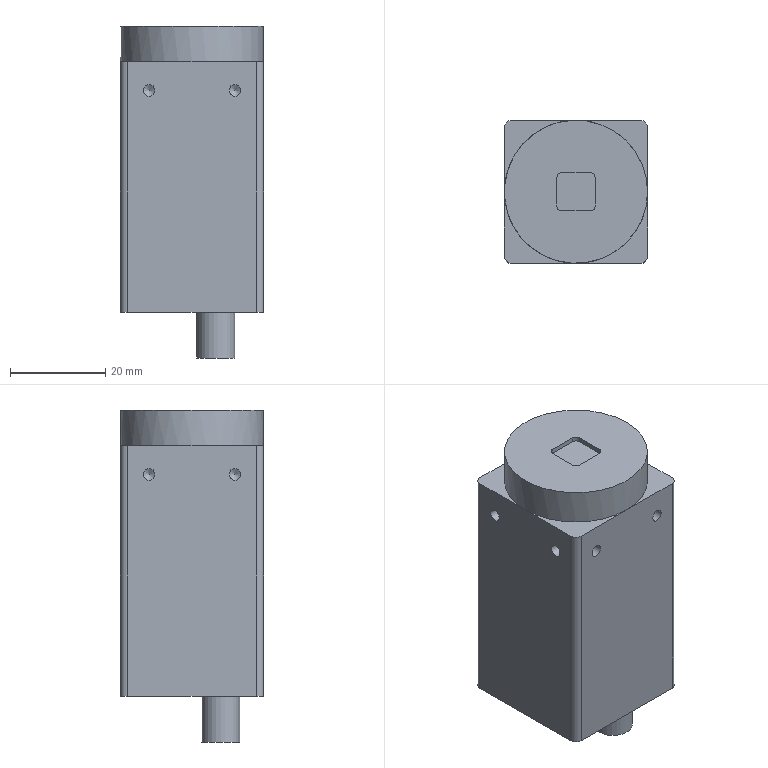Part | NX | 1 solid | 56 faces | box 30 x 30 x 69.6 mm | volume 52533 mm3 | cylinder 29 | plane 16 | cone 11 | commonest cylinder face diameters 2.5 x16 2 x4 3 x4 2.05 x3 8 x1 30 x1
STEP:
#1=CARTESIAN_POINT('',(9.,-15.,45.25));
#2=VERTEX_POINT('',#1);
#3=CARTESIAN_POINT('',(9.,-15.,46.5));
#4=DIRECTION('',(0.,-1.,0.));
#5=DIRECTION('',(0.,0.,-1.));
#6=AXIS2_PLACEMENT_3D('',#3,#4,#5);
#7=CIRCLE('',#6,1.25);
#8=EDGE_CURVE('',#2,#2,#7,.T.);
#9=ORIENTED_EDGE('',*,*,#8,.T.);
#10=EDGE_LOOP('',(#9));
#11=FACE_BOUND('',#10,.T.);
#12=CARTESIAN_POINT('',(9.,-9.,47.75));
#13=VERTEX_POINT('',#12);
#14=CARTESIAN_POINT('',(9.,-9.,45.25));
#15=VERTEX_POINT('',#14);
#16=CARTESIAN_POINT('',(9.,-9.,46.5));
#17=DIRECTION('',(-0.7071,-0.7071,0.));
#18=DIRECTION('',(0.7071,-0.7071,0.));
#19=AXIS2_PLACEMENT_3D('',#16,#17,#18);
#20=ELLIPSE('',#19,1.768,1.25);
#21=EDGE_CURVE('',#13,#15,#20,.F.);
#22=ORIENTED_EDGE('',*,*,#21,.T.);
#23=CARTESIAN_POINT('',(9.,-9.,46.5));
#24=DIRECTION('',(0.7071,-0.7071,0.));
#25=DIRECTION('',(-0.7071,-0.7071,0.));
#26=AXIS2_PLACEMENT_3D('',#23,#24,#25);
#27=ELLIPSE('',#26,1.768,1.25);
#28=EDGE_CURVE('',#15,#13,#27,.F.);
#29=ORIENTED_EDGE('',*,*,#28,.T.);
#30=EDGE_LOOP('',(#22,#29));
#31=FACE_BOUND('',#30,.T.);
#32=CARTESIAN_POINT('',(9.,-15.,46.5));
#33=DIRECTION('',(0.,-1.,0.));
#34=DIRECTION('',(0.,0.,-1.));
#35=AXIS2_PLACEMENT_3D('',#32,#33,#34);
#36=CYLINDRICAL_SURFACE('',#35,1.25);
#37=ADVANCED_FACE('',(#11,#31),#36,.F.);
#38=CARTESIAN_POINT('',(9.,15.,47.75));
#39=VERTEX_POINT('',#38);
#40=CARTESIAN_POINT('',(9.,15.,46.5));
#41=DIRECTION('',(0.,1.,0.));
#42=DIRECTION('',(0.,0.,1.));
#43=AXIS2_PLACEMENT_3D('',#40,#41,#42);
#44=CIRCLE('',#43,1.25);
#45=EDGE_CURVE('',#39,#39,#44,.T.);
#46=ORIENTED_EDGE('',*,*,#45,.T.);
#47=EDGE_LOOP('',(#46));
#48=FACE_BOUND('',#47,.T.);
#49=CARTESIAN_POINT('',(9.,9.,45.25));
#50=VERTEX_POINT('',#49);
#51=CARTESIAN_POINT('',(9.,9.,47.75));
#52=VERTEX_POINT('',#51);
#53=CARTESIAN_POINT('',(9.,9.,46.5));
#54=DIRECTION('',(-0.7071,0.7071,0.));
#55=DIRECTION('',(0.7071,0.7071,0.));
#56=AXIS2_PLACEMENT_3D('',#53,#54,#55);
#57=ELLIPSE('',#56,1.768,1.25);
#58=EDGE_CURVE('',#50,#52,#57,.F.);
#59=ORIENTED_EDGE('',*,*,#58,.T.);
#60=CARTESIAN_POINT('',(9.,9.,46.5));
#61=DIRECTION('',(0.7071,0.7071,0.));
#62=DIRECTION('',(-0.7071,0.7071,0.));
#63=AXIS2_PLACEMENT_3D('',#60,#61,#62);
#64=ELLIPSE('',#63,1.768,1.25);
#65=EDGE_CURVE('',#52,#50,#64,.F.);
#66=ORIENTED_EDGE('',*,*,#65,.T.);
#67=EDGE_LOOP('',(#59,#66));
#68=FACE_BOUND('',#67,.T.);
#69=CARTESIAN_POINT('',(9.,15.,46.5));
#70=DIRECTION('',(0.,1.,0.));
#71=DIRECTION('',(0.,0.,1.));
#72=AXIS2_PLACEMENT_3D('',#69,#70,#71);
#73=CYLINDRICAL_SURFACE('',#72,1.25);
#74=ADVANCED_FACE('',(#48,#68),#73,.F.);
#75=CARTESIAN_POINT('',(-15.,9.,47.75));
#76=VERTEX_POINT('',#75);
#77=CARTESIAN_POINT('',(-15.,9.,46.5));
#78=DIRECTION('',(-1.,0.,0.));
#79=DIRECTION('',(0.,0.,1.));
#80=AXIS2_PLACEMENT_3D('',#77,#78,#79);
#81=CIRCLE('',#80,1.25);
#82=EDGE_CURVE('',#76,#76,#81,.T.);
#83=ORIENTED_EDGE('',*,*,#82,.T.);
#84=EDGE_LOOP('',(#83));
#85=FACE_BOUND('',#84,.T.);
#86=CARTESIAN_POINT('',(-9.,9.,45.25));
#87=VERTEX_POINT('',#86);
#88=CARTESIAN_POINT('',(-9.,9.,47.75));
#89=VERTEX_POINT('',#88);
#90=CARTESIAN_POINT('',(-9.,9.,46.5));
#91=DIRECTION('',(-0.7071,-0.7071,0.));
#92=DIRECTION('',(-0.7071,0.7071,0.));
#93=AXIS2_PLACEMENT_3D('',#90,#91,#92);
#94=ELLIPSE('',#93,1.768,1.25);
#95=EDGE_CURVE('',#87,#89,#94,.F.);
#96=ORIENTED_EDGE('',*,*,#95,.T.);
#97=CARTESIAN_POINT('',(-9.,9.,46.5));
#98=DIRECTION('',(-0.7071,0.7071,0.));
#99=DIRECTION('',(-0.7071,-0.7071,0.));
#100=AXIS2_PLACEMENT_3D('',#97,#98,#99);
#101=ELLIPSE('',#100,1.768,1.25);
#102=EDGE_CURVE('',#89,#87,#101,.F.);
#103=ORIENTED_EDGE('',*,*,#102,.T.);
#104=EDGE_LOOP('',(#96,#103));
#105=FACE_BOUND('',#104,.T.);
#106=CARTESIAN_POINT('',(-15.,9.,46.5));
#107=DIRECTION('',(-1.,0.,0.));
#108=DIRECTION('',(0.,0.,1.));
#109=AXIS2_PLACEMENT_3D('',#106,#107,#108);
#110=CYLINDRICAL_SURFACE('',#109,1.25);
#111=ADVANCED_FACE('',(#85,#105),#110,.F.);
#112=CARTESIAN_POINT('',(-9.,-15.,45.25));
#113=VERTEX_POINT('',#112);
#114=CARTESIAN_POINT('',(-9.,-15.,46.5));
#115=DIRECTION('',(0.,-1.,0.));
#116=DIRECTION('',(0.,0.,-1.));
#117=AXIS2_PLACEMENT_3D('',#114,#115,#116);
#118=CIRCLE('',#117,1.25);
#119=EDGE_CURVE('',#113,#113,#118,.T.);
#120=ORIENTED_EDGE('',*,*,#119,.T.);
#121=EDGE_LOOP('',(#120));
#122=FACE_BOUND('',#121,.T.);
#123=CARTESIAN_POINT('',(-9.,-9.,45.25));
#124=VERTEX_POINT('',#123);
#125=CARTESIAN_POINT('',(-9.,-9.,47.75));
#126=VERTEX_POINT('',#125);
#127=CARTESIAN_POINT('',(-9.,-9.,46.5));
#128=DIRECTION('',(0.7071,-0.7071,0.));
#129=DIRECTION('',(-0.7071,-0.7071,0.));
#130=AXIS2_PLACEMENT_3D('',#127,#128,#129);
#131=ELLIPSE('',#130,1.768,1.25);
#132=EDGE_CURVE('',#124,#126,#131,.F.);
#133=ORIENTED_EDGE('',*,*,#132,.T.);
#134=CARTESIAN_POINT('',(-9.,-9.,46.5));
#135=DIRECTION('',(-0.7071,-0.7071,0.));
#136=DIRECTION('',(0.7071,-0.7071,0.));
#137=AXIS2_PLACEMENT_3D('',#134,#135,#136);
#138=ELLIPSE('',#137,1.768,1.25);
#139=EDGE_CURVE('',#126,#124,#138,.F.);
#140=ORIENTED_EDGE('',*,*,#139,.T.);
#141=EDGE_LOOP('',(#133,#140));
#142=FACE_BOUND('',#141,.T.);
#143=CARTESIAN_POINT('',(-9.,-15.,46.5));
#144=DIRECTION('',(0.,-1.,0.));
#145=DIRECTION('',(0.,0.,-1.));
#146=AXIS2_PLACEMENT_3D('',#143,#144,#145);
#147=CYLINDRICAL_SURFACE('',#146,1.25);
#148=ADVANCED_FACE('',(#122,#142),#147,.F.);
#149=CARTESIAN_POINT('',(15.,0.,60.));
#150=VERTEX_POINT('',#149);
#151=CARTESIAN_POINT('',(0.,0.,60.));
#152=DIRECTION('',(0.,0.,1.));
#153=DIRECTION('',(1.,0.,0.));
#154=AXIS2_PLACEMENT_3D('',#151,#152,#153);
#155=CIRCLE('',#154,15.);
#156=EDGE_CURVE('',#150,#150,#155,.T.);
#157=ORIENTED_EDGE('',*,*,#156,.T.);
#158=EDGE_LOOP('',(#157));
#159=FACE_BOUND('',#158,.T.);
#160=CARTESIAN_POINT('',(-4.,-3.,60.));
#161=VERTEX_POINT('',#160);
#162=CARTESIAN_POINT('',(-4.,3.,60.));
#163=VERTEX_POINT('',#162);
#164=CARTESIAN_POINT('',(-4.,3.,60.));
#165=DIRECTION('',(0.,1.,0.));
#166=VECTOR('',#165,1000.);
#167=LINE('',#164,#166);
#168=EDGE_CURVE('',#161,#163,#167,.T.);
#169=ORIENTED_EDGE('',*,*,#168,.T.);
#170=CARTESIAN_POINT('',(-3.,4.,60.));
#171=VERTEX_POINT('',#170);
#172=CARTESIAN_POINT('',(-3.,3.,60.));
#173=DIRECTION('',(0.,0.,-1.));
#174=DIRECTION('',(-1.,0.,0.));
#175=AXIS2_PLACEMENT_3D('',#172,#173,#174);
#176=CIRCLE('',#175,1.);
#177=EDGE_CURVE('',#163,#171,#176,.T.);
#178=ORIENTED_EDGE('',*,*,#177,.T.);
#179=CARTESIAN_POINT('',(3.,4.,60.));
#180=VERTEX_POINT('',#179);
#181=CARTESIAN_POINT('',(3.,4.,60.));
#182=DIRECTION('',(1.,0.,0.));
#183=VECTOR('',#182,1000.);
#184=LINE('',#181,#183);
#185=EDGE_CURVE('',#171,#180,#184,.T.);
#186=ORIENTED_EDGE('',*,*,#185,.T.);
#187=CARTESIAN_POINT('',(4.,3.,60.));
#188=VERTEX_POINT('',#187);
#189=CARTESIAN_POINT('',(3.,3.,60.));
#190=DIRECTION('',(0.,0.,-1.));
#191=DIRECTION('',(-1.,0.,0.));
#192=AXIS2_PLACEMENT_3D('',#189,#190,#191);
#193=CIRCLE('',#192,1.);
#194=EDGE_CURVE('',#180,#188,#193,.T.);
#195=ORIENTED_EDGE('',*,*,#194,.T.);
#196=CARTESIAN_POINT('',(4.,-3.,60.));
#197=VERTEX_POINT('',#196);
#198=CARTESIAN_POINT('',(4.,3.,60.));
#199=DIRECTION('',(0.,-1.,0.));
#200=VECTOR('',#199,1000.);
#201=LINE('',#198,#200);
#202=EDGE_CURVE('',#188,#197,#201,.T.);
#203=ORIENTED_EDGE('',*,*,#202,.T.);
#204=CARTESIAN_POINT('',(3.,-4.,60.));
#205=VERTEX_POINT('',#204);
#206=CARTESIAN_POINT('',(3.,-3.,60.));
#207=DIRECTION('',(0.,0.,-1.));
#208=DIRECTION('',(-1.,0.,0.));
#209=AXIS2_PLACEMENT_3D('',#206,#207,#208);
#210=CIRCLE('',#209,1.);
#211=EDGE_CURVE('',#197,#205,#210,.T.);
#212=ORIENTED_EDGE('',*,*,#211,.T.);
#213=CARTESIAN_POINT('',(-3.,-4.,60.));
#214=VERTEX_POINT('',#213);
#215=CARTESIAN_POINT('',(3.,-4.,60.));
#216=DIRECTION('',(-1.,0.,0.));
#217=VECTOR('',#216,1000.);
#218=LINE('',#215,#217);
#219=EDGE_CURVE('',#205,#214,#218,.T.);
#220=ORIENTED_EDGE('',*,*,#219,.T.);
#221=CARTESIAN_POINT('',(-3.,-3.,60.));
#222=DIRECTION('',(0.,0.,-1.));
#223=DIRECTION('',(-1.,0.,0.));
#224=AXIS2_PLACEMENT_3D('',#221,#222,#223);
#225=CIRCLE('',#224,1.);
#226=EDGE_CURVE('',#214,#161,#225,.T.);
#227=ORIENTED_EDGE('',*,*,#226,.T.);
#228=EDGE_LOOP('',(#169,#178,#186,#195,#203,#212,#220,#227));
#229=FACE_BOUND('',#228,.T.);
#230=CARTESIAN_POINT('',(0.,0.,60.));
#231=DIRECTION('',(0.,0.,1.));
#232=DIRECTION('',(1.,0.,0.));
#233=AXIS2_PLACEMENT_3D('',#230,#231,#232);
#234=PLANE('',#233);
#235=ADVANCED_FACE('',(#159,#229),#234,.T.);
#236=CARTESIAN_POINT('',(13.5,-15.,0.));
#237=VERTEX_POINT('',#236);
#238=CARTESIAN_POINT('',(15.,-13.5,0.));
#239=VERTEX_POINT('',#238);
#240=CARTESIAN_POINT('',(13.5,-13.5,0.));
#241=DIRECTION('',(0.,0.,1.));
#242=DIRECTION('',(1.,0.,0.));
#243=AXIS2_PLACEMENT_3D('',#240,#241,#242);
#244=CIRCLE('',#243,1.5);
#245=EDGE_CURVE('',#237,#239,#244,.T.);
#246=ORIENTED_EDGE('',*,*,#245,.F.);
#247=CARTESIAN_POINT('',(-13.5,-15.,0.));
#248=VERTEX_POINT('',#247);
#249=CARTESIAN_POINT('',(-13.5,-15.,0.));
#250=DIRECTION('',(1.,0.,0.));
#251=VECTOR('',#250,1000.);
#252=LINE('',#249,#251);
#253=EDGE_CURVE('',#248,#237,#252,.T.);
#254=ORIENTED_EDGE('',*,*,#253,.F.);
#255=CARTESIAN_POINT('',(-15.,-13.5,0.));
#256=VERTEX_POINT('',#255);
#257=CARTESIAN_POINT('',(-13.5,-13.5,0.));
#258=DIRECTION('',(0.,0.,1.));
#259=DIRECTION('',(1.,0.,0.));
#260=AXIS2_PLACEMENT_3D('',#257,#258,#259);
#261=CIRCLE('',#260,1.5);
#262=EDGE_CURVE('',#256,#248,#261,.T.);
#263=ORIENTED_EDGE('',*,*,#262,.F.);
#264=CARTESIAN_POINT('',(-15.,13.5,0.));
#265=VERTEX_POINT('',#264);
#266=CARTESIAN_POINT('',(-15.,-13.5,0.));
#267=DIRECTION('',(0.,-1.,0.));
#268=VECTOR('',#267,1000.);
#269=LINE('',#266,#268);
#270=EDGE_CURVE('',#265,#256,#269,.T.);
#271=ORIENTED_EDGE('',*,*,#270,.F.);
#272=CARTESIAN_POINT('',(-13.5,15.,0.));
#273=VERTEX_POINT('',#272);
#274=CARTESIAN_POINT('',(-13.5,13.5,0.));
#275=DIRECTION('',(0.,0.,1.));
#276=DIRECTION('',(1.,0.,0.));
#277=AXIS2_PLACEMENT_3D('',#274,#275,#276);
#278=CIRCLE('',#277,1.5);
#279=EDGE_CURVE('',#273,#265,#278,.T.);
#280=ORIENTED_EDGE('',*,*,#279,.F.);
#281=CARTESIAN_POINT('',(13.5,15.,0.));
#282=VERTEX_POINT('',#281);
#283=CARTESIAN_POINT('',(-13.5,15.,0.));
#284=DIRECTION('',(-1.,0.,0.));
#285=VECTOR('',#284,1000.);
#286=LINE('',#283,#285);
#287=EDGE_CURVE('',#282,#273,#286,.T.);
#288=ORIENTED_EDGE('',*,*,#287,.F.);
#289=CARTESIAN_POINT('',(15.,13.5,0.));
#290=VERTEX_POINT('',#289);
#291=CARTESIAN_POINT('',(13.5,13.5,0.));
#292=DIRECTION('',(0.,0.,1.));
#293=DIRECTION('',(1.,0.,0.));
#294=AXIS2_PLACEMENT_3D('',#291,#292,#293);
#295=CIRCLE('',#294,1.5);
#296=EDGE_CURVE('',#290,#282,#295,.T.);
#297=ORIENTED_EDGE('',*,*,#296,.F.);
#298=CARTESIAN_POINT('',(15.,-13.5,0.));
#299=DIRECTION('',(0.,1.,0.));
#300=VECTOR('',#299,1000.);
#301=LINE('',#298,#300);
#302=EDGE_CURVE('',#239,#290,#301,.T.);
#303=ORIENTED_EDGE('',*,*,#302,.F.);
#304=EDGE_LOOP('',(#246,#254,#263,#271,#280,#288,#297,#303));
#305=FACE_BOUND('',#304,.T.);
#306=CARTESIAN_POINT('',(9.,-6.,0.));
#307=VERTEX_POINT('',#306);
#308=CARTESIAN_POINT('',(5.,-6.,0.));
#309=DIRECTION('',(0.,0.,1.));
#310=DIRECTION('',(1.,0.,0.));
#311=AXIS2_PLACEMENT_3D('',#308,#309,#310);
#312=CIRCLE('',#311,4.);
#313=EDGE_CURVE('',#307,#307,#312,.F.);
#314=ORIENTED_EDGE('',*,*,#313,.F.);
#315=EDGE_LOOP('',(#314));
#316=FACE_BOUND('',#315,.T.);
#317=CARTESIAN_POINT('',(13.5,-13.5,0.));
#318=DIRECTION('',(0.,0.,1.));
#319=DIRECTION('',(1.,0.,0.));
#320=AXIS2_PLACEMENT_3D('',#317,#318,#319);
#321=PLANE('',#320);
#322=ADVANCED_FACE('',(#305,#316),#321,.F.);
#323=CARTESIAN_POINT('',(15.,0.,52.5));
#324=VERTEX_POINT('',#323);
#325=CARTESIAN_POINT('',(0.,15.,52.5));
#326=VERTEX_POINT('',#325);
#327=CARTESIAN_POINT('',(0.,0.,52.5));
#328=DIRECTION('',(0.,0.,1.));
#329=DIRECTION('',(1.,0.,0.));
#330=AXIS2_PLACEMENT_3D('',#327,#328,#329);
#331=CIRCLE('',#330,15.);
#332=EDGE_CURVE('',#324,#326,#331,.T.);
#333=ORIENTED_EDGE('',*,*,#332,.F.);
#334=CARTESIAN_POINT('',(15.,13.5,52.5));
#335=VERTEX_POINT('',#334);
#336=CARTESIAN_POINT('',(15.,-13.5,52.5));
#337=DIRECTION('',(0.,1.,0.));
#338=VECTOR('',#337,1000.);
#339=LINE('',#336,#338);
#340=EDGE_CURVE('',#324,#335,#339,.T.);
#341=ORIENTED_EDGE('',*,*,#340,.T.);
#342=CARTESIAN_POINT('',(13.5,15.,52.5));
#343=VERTEX_POINT('',#342);
#344=CARTESIAN_POINT('',(13.5,13.5,52.5));
#345=DIRECTION('',(0.,0.,1.));
#346=DIRECTION('',(1.,0.,0.));
#347=AXIS2_PLACEMENT_3D('',#344,#345,#346);
#348=CIRCLE('',#347,1.5);
#349=EDGE_CURVE('',#335,#343,#348,.T.);
#350=ORIENTED_EDGE('',*,*,#349,.T.);
#351=CARTESIAN_POINT('',(-13.5,15.,52.5));
#352=DIRECTION('',(-1.,0.,0.));
#353=VECTOR('',#352,1000.);
#354=LINE('',#351,#353);
#355=EDGE_CURVE('',#343,#326,#354,.T.);
#356=ORIENTED_EDGE('',*,*,#355,.T.);
#357=EDGE_LOOP('',(#333,#341,#350,#356));
#358=FACE_BOUND('',#357,.T.);
#359=CARTESIAN_POINT('',(13.5,-13.5,52.5));
#360=DIRECTION('',(0.,0.,1.));
#361=DIRECTION('',(1.,0.,0.));
#362=AXIS2_PLACEMENT_3D('',#359,#360,#361);
#363=PLANE('',#362);
#364=ADVANCED_FACE('',(#358),#363,.T.);
#365=CARTESIAN_POINT('',(-15.,0.,52.5));
#366=VERTEX_POINT('',#365);
#367=CARTESIAN_POINT('',(0.,0.,52.5));
#368=DIRECTION('',(0.,0.,1.));
#369=DIRECTION('',(1.,0.,0.));
#370=AXIS2_PLACEMENT_3D('',#367,#368,#369);
#371=CIRCLE('',#370,15.);
#372=EDGE_CURVE('',#326,#366,#371,.T.);
#373=ORIENTED_EDGE('',*,*,#372,.F.);
#374=CARTESIAN_POINT('',(-13.5,15.,52.5));
#375=VERTEX_POINT('',#374);
#376=CARTESIAN_POINT('',(-13.5,15.,52.5));
#377=DIRECTION('',(-1.,0.,0.));
#378=VECTOR('',#377,1000.);
#379=LINE('',#376,#378);
#380=EDGE_CURVE('',#326,#375,#379,.T.);
#381=ORIENTED_EDGE('',*,*,#380,.T.);
#382=CARTESIAN_POINT('',(-15.,13.5,52.5));
#383=VERTEX_POINT('',#382);
#384=CARTESIAN_POINT('',(-13.5,13.5,52.5));
#385=DIRECTION('',(0.,0.,1.));
#386=DIRECTION('',(1.,0.,0.));
#387=AXIS2_PLACEMENT_3D('',#384,#385,#386);
#388=CIRCLE('',#387,1.5);
#389=EDGE_CURVE('',#375,#383,#388,.T.);
#390=ORIENTED_EDGE('',*,*,#389,.T.);
#391=CARTESIAN_POINT('',(-15.,-13.5,52.5));
#392=DIRECTION('',(0.,-1.,0.));
#393=VECTOR('',#392,1000.);
#394=LINE('',#391,#393);
#395=EDGE_CURVE('',#383,#366,#394,.T.);
#396=ORIENTED_EDGE('',*,*,#395,.T.);
#397=EDGE_LOOP('',(#373,#381,#390,#396));
#398=FACE_BOUND('',#397,.T.);
#399=CARTESIAN_POINT('',(13.5,-13.5,52.5));
#400=DIRECTION('',(0.,0.,1.));
#401=DIRECTION('',(1.,0.,0.));
#402=AXIS2_PLACEMENT_3D('',#399,#400,#401);
#403=PLANE('',#402);
#404=ADVANCED_FACE('',(#398),#403,.T.);
#405=CARTESIAN_POINT('',(0.,-15.,52.5));
#406=VERTEX_POINT('',#405);
#407=CARTESIAN_POINT('',(0.,0.,52.5));
#408=DIRECTION('',(0.,0.,1.));
#409=DIRECTION('',(1.,0.,0.));
#410=AXIS2_PLACEMENT_3D('',#407,#408,#409);
#411=CIRCLE('',#410,15.);
#412=EDGE_CURVE('',#366,#406,#411,.T.);
#413=ORIENTED_EDGE('',*,*,#412,.F.);
#414=CARTESIAN_POINT('',(-15.,-13.5,52.5));
#415=VERTEX_POINT('',#414);
#416=CARTESIAN_POINT('',(-15.,-13.5,52.5));
#417=DIRECTION('',(0.,-1.,0.));
#418=VECTOR('',#417,1000.);
#419=LINE('',#416,#418);
#420=EDGE_CURVE('',#366,#415,#419,.T.);
#421=ORIENTED_EDGE('',*,*,#420,.T.);
#422=CARTESIAN_POINT('',(-13.5,-15.,52.5));
#423=VERTEX_POINT('',#422);
#424=CARTESIAN_POINT('',(-13.5,-13.5,52.5));
#425=DIRECTION('',(0.,0.,1.));
#426=DIRECTION('',(1.,0.,0.));
#427=AXIS2_PLACEMENT_3D('',#424,#425,#426);
#428=CIRCLE('',#427,1.5);
#429=EDGE_CURVE('',#415,#423,#428,.T.);
#430=ORIENTED_EDGE('',*,*,#429,.T.);
#431=CARTESIAN_POINT('',(-13.5,-15.,52.5));
#432=DIRECTION('',(1.,0.,0.));
#433=VECTOR('',#432,1000.);
#434=LINE('',#431,#433);
#435=EDGE_CURVE('',#423,#406,#434,.T.);
#436=ORIENTED_EDGE('',*,*,#435,.T.);
#437=EDGE_LOOP('',(#413,#421,#430,#436));
#438=FACE_BOUND('',#437,.T.);
#439=CARTESIAN_POINT('',(13.5,-13.5,52.5));
#440=DIRECTION('',(0.,0.,1.));
#441=DIRECTION('',(1.,0.,0.));
#442=AXIS2_PLACEMENT_3D('',#439,#440,#441);
#443=PLANE('',#442);
#444=ADVANCED_FACE('',(#438),#443,.T.);
#445=ORIENTED_EDGE('',*,*,#245,.T.);
#446=CARTESIAN_POINT('',(15.,-13.5,52.5));
#447=VERTEX_POINT('',#446);
#448=CARTESIAN_POINT('',(15.,-13.5,52.5));
#449=DIRECTION('',(0.,0.,-1.));
#450=VECTOR('',#449,1000.);
#451=LINE('',#448,#450);
#452=EDGE_CURVE('',#447,#239,#451,.T.);
#453=ORIENTED_EDGE('',*,*,#452,.F.);
#454=CARTESIAN_POINT('',(13.5,-15.,52.5));
#455=VERTEX_POINT('',#454);
#456=CARTESIAN_POINT('',(13.5,-13.5,52.5));
#457=DIRECTION('',(0.,0.,1.));
#458=DIRECTION('',(1.,0.,0.));
#459=AXIS2_PLACEMENT_3D('',#456,#457,#458);
#460=CIRCLE('',#459,1.5);
#461=EDGE_CURVE('',#455,#447,#460,.T.);
#462=ORIENTED_EDGE('',*,*,#461,.F.);
#463=CARTESIAN_POINT('',(13.5,-15.,52.5));
#464=DIRECTION('',(0.,0.,-1.));
#465=VECTOR('',#464,1000.);
#466=LINE('',#463,#465);
#467=EDGE_CURVE('',#455,#237,#466,.T.);
#468=ORIENTED_EDGE('',*,*,#467,.T.);
#469=EDGE_LOOP('',(#445,#453,#462,#468));
#470=FACE_BOUND('',#469,.T.);
#471=CARTESIAN_POINT('',(13.5,-13.5,52.5));
#472=DIRECTION('',(0.,0.,-1.));
#473=DIRECTION('',(-1.,0.,0.));
#474=AXIS2_PLACEMENT_3D('',#471,#472,#473);
#475=CYLINDRICAL_SURFACE('',#474,1.5);
#476=ADVANCED_FACE('',(#470),#475,.T.);
#477=CARTESIAN_POINT('',(15.,-9.,45.25));
#478=VERTEX_POINT('',#477);
#479=CARTESIAN_POINT('',(15.,-9.,46.5));
#480=DIRECTION('',(1.,0.,0.));
#481=DIRECTION('',(0.,0.,-1.));
#482=AXIS2_PLACEMENT_3D('',#479,#480,#481);
#483=CIRCLE('',#482,1.25);
#484=EDGE_CURVE('',#478,#478,#483,.T.);
#485=ORIENTED_EDGE('',*,*,#484,.F.);
#486=EDGE_LOOP('',(#485));
#487=FACE_BOUND('',#486,.T.);
#488=CARTESIAN_POINT('',(15.,9.,45.25));
#489=VERTEX_POINT('',#488);
#490=CARTESIAN_POINT('',(15.,9.,46.5));
#491=DIRECTION('',(1.,0.,0.));
#492=DIRECTION('',(0.,0.,-1.));
#493=AXIS2_PLACEMENT_3D('',#490,#491,#492);
#494=CIRCLE('',#493,1.25);
#495=EDGE_CURVE('',#489,#489,#494,.T.);
#496=ORIENTED_EDGE('',*,*,#495,.F.);
#497=EDGE_LOOP('',(#496));
#498=FACE_BOUND('',#497,.T.);
#499=ORIENTED_EDGE('',*,*,#302,.T.);
#500=CARTESIAN_POINT('',(15.,13.5,52.5));
#501=DIRECTION('',(0.,0.,-1.));
#502=VECTOR('',#501,1000.);
#503=LINE('',#500,#502);
#504=EDGE_CURVE('',#335,#290,#503,.T.);
#505=ORIENTED_EDGE('',*,*,#504,.F.);
#506=ORIENTED_EDGE('',*,*,#340,.F.);
#507=CARTESIAN_POINT('',(15.,-13.5,52.5));
#508=DIRECTION('',(0.,1.,0.));
#509=VECTOR('',#508,1000.);
#510=LINE('',#507,#509);
#511=EDGE_CURVE('',#447,#324,#510,.T.);
#512=ORIENTED_EDGE('',*,*,#511,.F.);
#513=ORIENTED_EDGE('',*,*,#452,.T.);
#514=EDGE_LOOP('',(#499,#505,#506,#512,#513));
#515=FACE_BOUND('',#514,.T.);
#516=CARTESIAN_POINT('',(15.,-13.5,52.5));
#517=DIRECTION('',(-1.,0.,0.));
#518=DIRECTION('',(0.,-1.,0.));
#519=AXIS2_PLACEMENT_3D('',#516,#517,#518);
#520=PLANE('',#519);
#521=ADVANCED_FACE('',(#487,#498,#515),#520,.F.);
#522=ORIENTED_EDGE('',*,*,#296,.T.);
#523=CARTESIAN_POINT('',(13.5,15.,52.5));
#524=DIRECTION('',(0.,0.,-1.));
#525=VECTOR('',#524,1000.);
#526=LINE('',#523,#525);
#527=EDGE_CURVE('',#343,#282,#526,.T.);
#528=ORIENTED_EDGE('',*,*,#527,.F.);
#529=ORIENTED_EDGE('',*,*,#349,.F.);
#530=ORIENTED_EDGE('',*,*,#504,.T.);
#531=EDGE_LOOP('',(#522,#528,#529,#530));
#532=FACE_BOUND('',#531,.T.);
#533=CARTESIAN_POINT('',(13.5,13.5,52.5));
#534=DIRECTION('',(0.,0.,-1.));
#535=DIRECTION('',(-1.,0.,0.));
#536=AXIS2_PLACEMENT_3D('',#533,#534,#535);
#537=CYLINDRICAL_SURFACE('',#536,1.5);
#538=ADVANCED_FACE('',(#532),#537,.T.);
#539=CARTESIAN_POINT('',(0.,15.,47.525));
#540=VERTEX_POINT('',#539);
#541=CARTESIAN_POINT('',(0.,15.,46.5));
#542=DIRECTION('',(0.,1.,0.));
#543=DIRECTION('',(0.,0.,1.));
#544=AXIS2_PLACEMENT_3D('',#541,#542,#543);
#545=CIRCLE('',#544,1.025);
#546=EDGE_CURVE('',#540,#540,#545,.T.);
#547=ORIENTED_EDGE('',*,*,#546,.F.);
#548=EDGE_LOOP('',(#547));
#549=FACE_BOUND('',#548,.T.);
#550=CARTESIAN_POINT('',(-11.5,15.,16.525));
#551=VERTEX_POINT('',#550);
#552=CARTESIAN_POINT('',(-11.5,15.,15.5));
#553=DIRECTION('',(0.,1.,0.));
#554=DIRECTION('',(0.,0.,1.));
#555=AXIS2_PLACEMENT_3D('',#552,#553,#554);
#556=CIRCLE('',#555,1.025);
#557=EDGE_CURVE('',#551,#551,#556,.T.);
#558=ORIENTED_EDGE('',*,*,#557,.F.);
#559=EDGE_LOOP('',(#558));
#560=FACE_BOUND('',#559,.T.);
#561=CARTESIAN_POINT('',(11.5,15.,16.525));
#562=VERTEX_POINT('',#561);
#563=CARTESIAN_POINT('',(11.5,15.,15.5));
#564=DIRECTION('',(0.,1.,0.));
#565=DIRECTION('',(0.,0.,1.));
#566=AXIS2_PLACEMENT_3D('',#563,#564,#565);
#567=CIRCLE('',#566,1.025);
#568=EDGE_CURVE('',#562,#562,#567,.T.);
#569=ORIENTED_EDGE('',*,*,#568,.F.);
#570=EDGE_LOOP('',(#569));
#571=FACE_BOUND('',#570,.T.);
#572=ORIENTED_EDGE('',*,*,#45,.F.);
#573=EDGE_LOOP('',(#572));
#574=FACE_BOUND('',#573,.T.);
#575=CARTESIAN_POINT('',(-9.,15.,47.75));
#576=VERTEX_POINT('',#575);
#577=CARTESIAN_POINT('',(-9.,15.,46.5));
#578=DIRECTION('',(0.,1.,0.));
#579=DIRECTION('',(0.,0.,1.));
#580=AXIS2_PLACEMENT_3D('',#577,#578,#579);
#581=CIRCLE('',#580,1.25);
#582=EDGE_CURVE('',#576,#576,#581,.T.);
#583=ORIENTED_EDGE('',*,*,#582,.F.);
#584=EDGE_LOOP('',(#583));
#585=FACE_BOUND('',#584,.T.);
#586=ORIENTED_EDGE('',*,*,#287,.T.);
#587=CARTESIAN_POINT('',(-13.5,15.,52.5));
#588=DIRECTION('',(0.,0.,-1.));
#589=VECTOR('',#588,1000.);
#590=LINE('',#587,#589);
#591=EDGE_CURVE('',#375,#273,#590,.T.);
#592=ORIENTED_EDGE('',*,*,#591,.F.);
#593=ORIENTED_EDGE('',*,*,#380,.F.);
#594=ORIENTED_EDGE('',*,*,#355,.F.);
#595=ORIENTED_EDGE('',*,*,#527,.T.);
#596=EDGE_LOOP('',(#586,#592,#593,#594,#595));
#597=FACE_BOUND('',#596,.T.);
#598=CARTESIAN_POINT('',(-13.5,15.,52.5));
#599=DIRECTION('',(0.,-1.,0.));
#600=DIRECTION('',(0.,0.,-1.));
#601=AXIS2_PLACEMENT_3D('',#598,#599,#600);
#602=PLANE('',#601);
#603=ADVANCED_FACE('',(#549,#560,#571,#574,#585,#597),#602,.F.);
#604=ORIENTED_EDGE('',*,*,#279,.T.);
#605=CARTESIAN_POINT('',(-15.,13.5,52.5));
#606=DIRECTION('',(0.,0.,-1.));
#607=VECTOR('',#606,1000.);
#608=LINE('',#605,#607);
#609=EDGE_CURVE('',#383,#265,#608,.T.);
#610=ORIENTED_EDGE('',*,*,#609,.F.);
#611=ORIENTED_EDGE('',*,*,#389,.F.);
#612=ORIENTED_EDGE('',*,*,#591,.T.);
#613=EDGE_LOOP('',(#604,#610,#611,#612));
#614=FACE_BOUND('',#613,.T.);
#615=CARTESIAN_POINT('',(-13.5,13.5,52.5));
#616=DIRECTION('',(0.,0.,-1.));
#617=DIRECTION('',(-1.,0.,0.));
#618=AXIS2_PLACEMENT_3D('',#615,#616,#617);
#619=CYLINDRICAL_SURFACE('',#618,1.5);
#620=ADVANCED_FACE('',(#614),#619,.T.);
#621=ORIENTED_EDGE('',*,*,#82,.F.);
#622=EDGE_LOOP('',(#621));
#623=FACE_BOUND('',#622,.T.);
#624=CARTESIAN_POINT('',(-15.,-9.,47.75));
#625=VERTEX_POINT('',#624);
#626=CARTESIAN_POINT('',(-15.,-9.,46.5));
#627=DIRECTION('',(-1.,0.,0.));
#628=DIRECTION('',(0.,0.,1.));
#629=AXIS2_PLACEMENT_3D('',#626,#627,#628);
#630=CIRCLE('',#629,1.25);
#631=EDGE_CURVE('',#625,#625,#630,.T.);
#632=ORIENTED_EDGE('',*,*,#631,.F.);
#633=EDGE_LOOP('',(#632));
#634=FACE_BOUND('',#633,.T.);
#635=ORIENTED_EDGE('',*,*,#270,.T.);
#636=CARTESIAN_POINT('',(-15.,-13.5,52.5));
#637=DIRECTION('',(0.,0.,-1.));
#638=VECTOR('',#637,1000.);
#639=LINE('',#636,#638);
#640=EDGE_CURVE('',#415,#256,#639,.T.);
#641=ORIENTED_EDGE('',*,*,#640,.F.);
#642=ORIENTED_EDGE('',*,*,#420,.F.);
#643=ORIENTED_EDGE('',*,*,#395,.F.);
#644=ORIENTED_EDGE('',*,*,#609,.T.);
#645=EDGE_LOOP('',(#635,#641,#642,#643,#644));
#646=FACE_BOUND('',#645,.T.);
#647=CARTESIAN_POINT('',(-15.,-13.5,52.5));
#648=DIRECTION('',(1.,0.,0.));
#649=DIRECTION('',(0.,0.,-1.));
#650=AXIS2_PLACEMENT_3D('',#647,#648,#649);
#651=PLANE('',#650);
#652=ADVANCED_FACE('',(#623,#634,#646),#651,.F.);
#653=ORIENTED_EDGE('',*,*,#262,.T.);
#654=CARTESIAN_POINT('',(-13.5,-15.,52.5));
#655=DIRECTION('',(0.,0.,-1.));
#656=VECTOR('',#655,1000.);
#657=LINE('',#654,#656);
#658=EDGE_CURVE('',#423,#248,#657,.T.);
#659=ORIENTED_EDGE('',*,*,#658,.F.);
#660=ORIENTED_EDGE('',*,*,#429,.F.);
#661=ORIENTED_EDGE('',*,*,#640,.T.);
#662=EDGE_LOOP('',(#653,#659,#660,#661));
#663=FACE_BOUND('',#662,.T.);
#664=CARTESIAN_POINT('',(-13.5,-13.5,52.5));
#665=DIRECTION('',(0.,0.,-1.));
#666=DIRECTION('',(-1.,0.,0.));
#667=AXIS2_PLACEMENT_3D('',#664,#665,#666);
#668=CYLINDRICAL_SURFACE('',#667,1.5);
#669=ADVANCED_FACE('',(#663),#668,.T.);
#670=ORIENTED_EDGE('',*,*,#119,.F.);
#671=EDGE_LOOP('',(#670));
#672=FACE_BOUND('',#671,.T.);
#673=ORIENTED_EDGE('',*,*,#8,.F.);
#674=EDGE_LOOP('',(#673));
#675=FACE_BOUND('',#674,.T.);
#676=ORIENTED_EDGE('',*,*,#253,.T.);
#677=ORIENTED_EDGE('',*,*,#467,.F.);
#678=CARTESIAN_POINT('',(-13.5,-15.,52.5));
#679=DIRECTION('',(1.,0.,0.));
#680=VECTOR('',#679,1000.);
#681=LINE('',#678,#680);
#682=EDGE_CURVE('',#406,#455,#681,.T.);
#683=ORIENTED_EDGE('',*,*,#682,.F.);
#684=ORIENTED_EDGE('',*,*,#435,.F.);
#685=ORIENTED_EDGE('',*,*,#658,.T.);
#686=EDGE_LOOP('',(#676,#677,#683,#684,#685));
#687=FACE_BOUND('',#686,.T.);
#688=CARTESIAN_POINT('',(-13.5,-15.,52.5));
#689=DIRECTION('',(0.,1.,0.));
#690=DIRECTION('',(-1.,0.,0.));
#691=AXIS2_PLACEMENT_3D('',#688,#689,#690);
#692=PLANE('',#691);
#693=ADVANCED_FACE('',(#672,#675,#687),#692,.F.);
#694=CARTESIAN_POINT('',(0.,0.,52.5));
#695=DIRECTION('',(0.,0.,1.));
#696=DIRECTION('',(1.,0.,0.));
#697=AXIS2_PLACEMENT_3D('',#694,#695,#696);
#698=CIRCLE('',#697,15.);
#699=EDGE_CURVE('',#406,#324,#698,.T.);
#700=ORIENTED_EDGE('',*,*,#699,.F.);
#701=ORIENTED_EDGE('',*,*,#682,.T.);
#702=ORIENTED_EDGE('',*,*,#461,.T.);
#703=ORIENTED_EDGE('',*,*,#511,.T.);
#704=EDGE_LOOP('',(#700,#701,#702,#703));
#705=FACE_BOUND('',#704,.T.);
#706=CARTESIAN_POINT('',(13.5,-13.5,52.5));
#707=DIRECTION('',(0.,0.,1.));
#708=DIRECTION('',(1.,0.,0.));
#709=AXIS2_PLACEMENT_3D('',#706,#707,#708);
#710=PLANE('',#709);
#711=ADVANCED_FACE('',(#705),#710,.T.);
#712=ORIENTED_EDGE('',*,*,#156,.F.);
#713=EDGE_LOOP('',(#712));
#714=FACE_BOUND('',#713,.T.);
#715=ORIENTED_EDGE('',*,*,#332,.T.);
#716=ORIENTED_EDGE('',*,*,#372,.T.);
#717=ORIENTED_EDGE('',*,*,#412,.T.);
#718=ORIENTED_EDGE('',*,*,#699,.T.);
#719=EDGE_LOOP('',(#715,#716,#717,#718));
#720=FACE_BOUND('',#719,.T.);
#721=CARTESIAN_POINT('',(0.,0.,60.));
#722=DIRECTION('',(0.,0.,-1.));
#723=DIRECTION('',(-1.,0.,0.));
#724=AXIS2_PLACEMENT_3D('',#721,#722,#723);
#725=CYLINDRICAL_SURFACE('',#724,15.);
#726=ADVANCED_FACE('',(#714,#720),#725,.T.);
#727=CARTESIAN_POINT('',(1.,-6.,-9.6));
#728=VERTEX_POINT('',#727);
#729=CARTESIAN_POINT('',(5.,-6.,-9.6));
#730=DIRECTION('',(0.,0.,-1.));
#731=DIRECTION('',(-1.,0.,0.));
#732=AXIS2_PLACEMENT_3D('',#729,#730,#731);
#733=CIRCLE('',#732,4.);
#734=EDGE_CURVE('',#728,#728,#733,.T.);
#735=ORIENTED_EDGE('',*,*,#734,.F.);
#736=EDGE_LOOP('',(#735));
#737=FACE_BOUND('',#736,.T.);
#738=ORIENTED_EDGE('',*,*,#313,.T.);
#739=EDGE_LOOP('',(#738));
#740=FACE_BOUND('',#739,.T.);
#741=CARTESIAN_POINT('',(5.,-6.,-9.6));
#742=DIRECTION('',(0.,0.,1.));
#743=DIRECTION('',(1.,0.,0.));
#744=AXIS2_PLACEMENT_3D('',#741,#742,#743);
#745=CYLINDRICAL_SURFACE('',#744,4.);
#746=ADVANCED_FACE('',(#737,#740),#745,.T.);
#747=ORIENTED_EDGE('',*,*,#734,.T.);
#748=EDGE_LOOP('',(#747));
#749=FACE_BOUND('',#748,.T.);
#750=CARTESIAN_POINT('',(5.,-6.,-9.6));
#751=DIRECTION('',(0.,0.,-1.));
#752=DIRECTION('',(-1.,0.,0.));
#753=AXIS2_PLACEMENT_3D('',#750,#751,#752);
#754=PLANE('',#753);
#755=ADVANCED_FACE('',(#749),#754,.T.);
#756=ORIENTED_EDGE('',*,*,#177,.F.);
#757=CARTESIAN_POINT('',(-4.,3.,59.));
#758=VERTEX_POINT('',#757);
#759=CARTESIAN_POINT('',(-4.,3.,59.));
#760=DIRECTION('',(0.,0.,1.));
#761=VECTOR('',#760,1000.);
#762=LINE('',#759,#761);
#763=EDGE_CURVE('',#758,#163,#762,.T.);
#764=ORIENTED_EDGE('',*,*,#763,.F.);
#765=CARTESIAN_POINT('',(-3.,4.,59.));
#766=VERTEX_POINT('',#765);
#767=CARTESIAN_POINT('',(-3.,3.,59.));
#768=DIRECTION('',(0.,0.,-1.));
#769=DIRECTION('',(-1.,0.,0.));
#770=AXIS2_PLACEMENT_3D('',#767,#768,#769);
#771=CIRCLE('',#770,1.);
#772=EDGE_CURVE('',#758,#766,#771,.T.);
#773=ORIENTED_EDGE('',*,*,#772,.T.);
#774=CARTESIAN_POINT('',(-3.,4.,59.));
#775=DIRECTION('',(0.,0.,1.));
#776=VECTOR('',#775,1000.);
#777=LINE('',#774,#776);
#778=EDGE_CURVE('',#766,#171,#777,.T.);
#779=ORIENTED_EDGE('',*,*,#778,.T.);
#780=EDGE_LOOP('',(#756,#764,#773,#779));
#781=FACE_BOUND('',#780,.T.);
#782=CARTESIAN_POINT('',(-3.,3.,59.));
#783=DIRECTION('',(0.,0.,1.));
#784=DIRECTION('',(1.,0.,0.));
#785=AXIS2_PLACEMENT_3D('',#782,#783,#784);
#786=CYLINDRICAL_SURFACE('',#785,1.);
#787=ADVANCED_FACE('',(#781),#786,.F.);
#788=ORIENTED_EDGE('',*,*,#185,.F.);
#789=ORIENTED_EDGE('',*,*,#778,.F.);
#790=CARTESIAN_POINT('',(3.,4.,59.));
#791=VERTEX_POINT('',#790);
#792=CARTESIAN_POINT('',(3.,4.,59.));
#793=DIRECTION('',(1.,0.,0.));
#794=VECTOR('',#793,1000.);
#795=LINE('',#792,#794);
#796=EDGE_CURVE('',#766,#791,#795,.T.);
#797=ORIENTED_EDGE('',*,*,#796,.T.);
#798=CARTESIAN_POINT('',(3.,4.,59.));
#799=DIRECTION('',(0.,0.,1.));
#800=VECTOR('',#799,1000.);
#801=LINE('',#798,#800);
#802=EDGE_CURVE('',#791,#180,#801,.T.);
#803=ORIENTED_EDGE('',*,*,#802,.T.);
#804=EDGE_LOOP('',(#788,#789,#797,#803));
#805=FACE_BOUND('',#804,.T.);
#806=CARTESIAN_POINT('',(3.,4.,59.));
#807=DIRECTION('',(0.,-1.,0.));
#808=DIRECTION('',(0.,0.,-1.));
#809=AXIS2_PLACEMENT_3D('',#806,#807,#808);
#810=PLANE('',#809);
#811=ADVANCED_FACE('',(#805),#810,.T.);
#812=ORIENTED_EDGE('',*,*,#194,.F.);
#813=ORIENTED_EDGE('',*,*,#802,.F.);
#814=CARTESIAN_POINT('',(4.,3.,59.));
#815=VERTEX_POINT('',#814);
#816=CARTESIAN_POINT('',(3.,3.,59.));
#817=DIRECTION('',(0.,0.,-1.));
#818=DIRECTION('',(-1.,0.,0.));
#819=AXIS2_PLACEMENT_3D('',#816,#817,#818);
#820=CIRCLE('',#819,1.);
#821=EDGE_CURVE('',#791,#815,#820,.T.);
#822=ORIENTED_EDGE('',*,*,#821,.T.);
#823=CARTESIAN_POINT('',(4.,3.,59.));
#824=DIRECTION('',(0.,0.,1.));
#825=VECTOR('',#824,1000.);
#826=LINE('',#823,#825);
#827=EDGE_CURVE('',#815,#188,#826,.T.);
#828=ORIENTED_EDGE('',*,*,#827,.T.);
#829=EDGE_LOOP('',(#812,#813,#822,#828));
#830=FACE_BOUND('',#829,.T.);
#831=CARTESIAN_POINT('',(3.,3.,59.));
#832=DIRECTION('',(0.,0.,1.));
#833=DIRECTION('',(1.,0.,0.));
#834=AXIS2_PLACEMENT_3D('',#831,#832,#833);
#835=CYLINDRICAL_SURFACE('',#834,1.);
#836=ADVANCED_FACE('',(#830),#835,.F.);
#837=ORIENTED_EDGE('',*,*,#202,.F.);
#838=ORIENTED_EDGE('',*,*,#827,.F.);
#839=CARTESIAN_POINT('',(4.,-3.,59.));
#840=VERTEX_POINT('',#839);
#841=CARTESIAN_POINT('',(4.,3.,59.));
#842=DIRECTION('',(0.,-1.,0.));
#843=VECTOR('',#842,1000.);
#844=LINE('',#841,#843);
#845=EDGE_CURVE('',#815,#840,#844,.T.);
#846=ORIENTED_EDGE('',*,*,#845,.T.);
#847=CARTESIAN_POINT('',(4.,-3.,59.));
#848=DIRECTION('',(0.,0.,1.));
#849=VECTOR('',#848,1000.);
#850=LINE('',#847,#849);
#851=EDGE_CURVE('',#840,#197,#850,.T.);
#852=ORIENTED_EDGE('',*,*,#851,.T.);
#853=EDGE_LOOP('',(#837,#838,#846,#852));
#854=FACE_BOUND('',#853,.T.);
#855=CARTESIAN_POINT('',(4.,3.,59.));
#856=DIRECTION('',(-1.,0.,0.));
#857=DIRECTION('',(0.,-1.,0.));
#858=AXIS2_PLACEMENT_3D('',#855,#856,#857);
#859=PLANE('',#858);
#860=ADVANCED_FACE('',(#854),#859,.T.);
#861=ORIENTED_EDGE('',*,*,#211,.F.);
#862=ORIENTED_EDGE('',*,*,#851,.F.);
#863=CARTESIAN_POINT('',(3.,-4.,59.));
#864=VERTEX_POINT('',#863);
#865=CARTESIAN_POINT('',(3.,-3.,59.));
#866=DIRECTION('',(0.,0.,-1.));
#867=DIRECTION('',(-1.,0.,0.));
#868=AXIS2_PLACEMENT_3D('',#865,#866,#867);
#869=CIRCLE('',#868,1.);
#870=EDGE_CURVE('',#840,#864,#869,.T.);
#871=ORIENTED_EDGE('',*,*,#870,.T.);
#872=CARTESIAN_POINT('',(3.,-4.,59.));
#873=DIRECTION('',(0.,0.,1.));
#874=VECTOR('',#873,1000.);
#875=LINE('',#872,#874);
#876=EDGE_CURVE('',#864,#205,#875,.T.);
#877=ORIENTED_EDGE('',*,*,#876,.T.);
#878=EDGE_LOOP('',(#861,#862,#871,#877));
#879=FACE_BOUND('',#878,.T.);
#880=CARTESIAN_POINT('',(3.,-3.,59.));
#881=DIRECTION('',(0.,0.,1.));
#882=DIRECTION('',(1.,0.,0.));
#883=AXIS2_PLACEMENT_3D('',#880,#881,#882);
#884=CYLINDRICAL_SURFACE('',#883,1.);
#885=ADVANCED_FACE('',(#879),#884,.F.);
#886=ORIENTED_EDGE('',*,*,#219,.F.);
#887=ORIENTED_EDGE('',*,*,#876,.F.);
#888=CARTESIAN_POINT('',(-3.,-4.,59.));
#889=VERTEX_POINT('',#888);
#890=CARTESIAN_POINT('',(3.,-4.,59.));
#891=DIRECTION('',(-1.,0.,0.));
#892=VECTOR('',#891,1000.);
#893=LINE('',#890,#892);
#894=EDGE_CURVE('',#864,#889,#893,.T.);
#895=ORIENTED_EDGE('',*,*,#894,.T.);
#896=CARTESIAN_POINT('',(-3.,-4.,59.));
#897=DIRECTION('',(0.,0.,1.));
#898=VECTOR('',#897,1000.);
#899=LINE('',#896,#898);
#900=EDGE_CURVE('',#889,#214,#899,.T.);
#901=ORIENTED_EDGE('',*,*,#900,.T.);
#902=EDGE_LOOP('',(#886,#887,#895,#901));
#903=FACE_BOUND('',#902,.T.);
#904=CARTESIAN_POINT('',(3.,-4.,59.));
#905=DIRECTION('',(0.,1.,0.));
#906=DIRECTION('',(0.,0.,1.));
#907=AXIS2_PLACEMENT_3D('',#904,#905,#906);
#908=PLANE('',#907);
#909=ADVANCED_FACE('',(#903),#908,.T.);
#910=ORIENTED_EDGE('',*,*,#226,.F.);
#911=ORIENTED_EDGE('',*,*,#900,.F.);
#912=CARTESIAN_POINT('',(-4.,-3.,59.));
#913=VERTEX_POINT('',#912);
#914=CARTESIAN_POINT('',(-3.,-3.,59.));
#915=DIRECTION('',(0.,0.,-1.));
#916=DIRECTION('',(-1.,0.,0.));
#917=AXIS2_PLACEMENT_3D('',#914,#915,#916);
#918=CIRCLE('',#917,1.);
#919=EDGE_CURVE('',#889,#913,#918,.T.);
#920=ORIENTED_EDGE('',*,*,#919,.T.);
#921=CARTESIAN_POINT('',(-4.,-3.,59.));
#922=DIRECTION('',(0.,0.,1.));
#923=VECTOR('',#922,1000.);
#924=LINE('',#921,#923);
#925=EDGE_CURVE('',#913,#161,#924,.T.);
#926=ORIENTED_EDGE('',*,*,#925,.T.);
#927=EDGE_LOOP('',(#910,#911,#920,#926));
#928=FACE_BOUND('',#927,.T.);
#929=CARTESIAN_POINT('',(-3.,-3.,59.));
#930=DIRECTION('',(0.,0.,1.));
#931=DIRECTION('',(1.,0.,0.));
#932=AXIS2_PLACEMENT_3D('',#929,#930,#931);
#933=CYLINDRICAL_SURFACE('',#932,1.);
#934=ADVANCED_FACE('',(#928),#933,.F.);
#935=ORIENTED_EDGE('',*,*,#168,.F.);
#936=ORIENTED_EDGE('',*,*,#925,.F.);
#937=CARTESIAN_POINT('',(-4.,3.,59.));
#938=DIRECTION('',(0.,1.,0.));
#939=VECTOR('',#938,1000.);
#940=LINE('',#937,#939);
#941=EDGE_CURVE('',#913,#758,#940,.T.);
#942=ORIENTED_EDGE('',*,*,#941,.T.);
#943=ORIENTED_EDGE('',*,*,#763,.T.);
#944=EDGE_LOOP('',(#935,#936,#942,#943));
#945=FACE_BOUND('',#944,.T.);
#946=CARTESIAN_POINT('',(-4.,3.,59.));
#947=DIRECTION('',(1.,0.,0.));
#948=DIRECTION('',(0.,1.,0.));
#949=AXIS2_PLACEMENT_3D('',#946,#947,#948);
#950=PLANE('',#949);
#951=ADVANCED_FACE('',(#945),#950,.T.);
#952=ORIENTED_EDGE('',*,*,#772,.F.);
#953=ORIENTED_EDGE('',*,*,#941,.F.);
#954=ORIENTED_EDGE('',*,*,#919,.F.);
#955=ORIENTED_EDGE('',*,*,#894,.F.);
#956=ORIENTED_EDGE('',*,*,#870,.F.);
#957=ORIENTED_EDGE('',*,*,#845,.F.);
#958=ORIENTED_EDGE('',*,*,#821,.F.);
#959=ORIENTED_EDGE('',*,*,#796,.F.);
#960=EDGE_LOOP('',(#952,#953,#954,#955,#956,#957,#958,#959));
#961=FACE_BOUND('',#960,.T.);
#962=CARTESIAN_POINT('',(-3.,3.,59.));
#963=DIRECTION('',(0.,0.,-1.));
#964=DIRECTION('',(-1.,0.,0.));
#965=AXIS2_PLACEMENT_3D('',#962,#963,#964);
#966=PLANE('',#965);
#967=ADVANCED_FACE('',(#961),#966,.F.);
#968=ORIENTED_EDGE('',*,*,#631,.T.);
#969=EDGE_LOOP('',(#968));
#970=FACE_BOUND('',#969,.T.);
#971=ORIENTED_EDGE('',*,*,#132,.F.);
#972=CARTESIAN_POINT('',(-9.,-9.,46.5));
#973=DIRECTION('',(-0.7071,-0.7071,0.));
#974=DIRECTION('',(0.7071,-0.7071,0.));
#975=AXIS2_PLACEMENT_3D('',#972,#973,#974);
#976=ELLIPSE('',#975,1.768,1.25);
#977=EDGE_CURVE('',#126,#124,#976,.T.);
#978=ORIENTED_EDGE('',*,*,#977,.F.);
#979=EDGE_LOOP('',(#971,#978));
#980=FACE_BOUND('',#979,.T.);
#981=CARTESIAN_POINT('',(-15.,-9.,46.5));
#982=DIRECTION('',(-1.,0.,0.));
#983=DIRECTION('',(0.,0.,1.));
#984=AXIS2_PLACEMENT_3D('',#981,#982,#983);
#985=CYLINDRICAL_SURFACE('',#984,1.25);
#986=ADVANCED_FACE('',(#970,#980),#985,.F.);
#987=CARTESIAN_POINT('',(-9.,-6.749,46.5));
#988=VERTEX_POINT('',#987);
#989=VERTEX_LOOP('',#988);
#990=FACE_BOUND('',#989,.T.);
#991=CARTESIAN_POINT('',(-9.,-7.5,45.25));
#992=VERTEX_POINT('',#991);
#993=CARTESIAN_POINT('',(-9.,-7.5,46.5));
#994=DIRECTION('',(0.,-1.,0.));
#995=DIRECTION('',(0.,0.,-1.));
#996=AXIS2_PLACEMENT_3D('',#993,#994,#995);
#997=CIRCLE('',#996,1.25);
#998=EDGE_CURVE('',#992,#992,#997,.T.);
#999=ORIENTED_EDGE('',*,*,#998,.T.);
#1000=EDGE_LOOP('',(#999));
#1001=FACE_BOUND('',#1000,.T.);
#1002=CARTESIAN_POINT('',(-9.,-7.5,46.5));
#1003=DIRECTION('',(0.,-1.,0.));
#1004=DIRECTION('',(0.,0.,-1.));
#1005=AXIS2_PLACEMENT_3D('',#1002,#1003,#1004);
#1006=CONICAL_SURFACE('',#1005,1.25,1.03);
#1007=ADVANCED_FACE('',(#990,#1001),#1006,.F.);
#1008=CARTESIAN_POINT('',(-9.,-9.,46.5));
#1009=DIRECTION('',(0.7071,-0.7071,0.));
#1010=DIRECTION('',(-0.7071,-0.7071,0.));
#1011=AXIS2_PLACEMENT_3D('',#1008,#1009,#1010);
#1012=ELLIPSE('',#1011,1.768,1.25);
#1013=EDGE_CURVE('',#124,#126,#1012,.T.);
#1014=ORIENTED_EDGE('',*,*,#1013,.T.);
#1015=ORIENTED_EDGE('',*,*,#977,.T.);
#1016=EDGE_LOOP('',(#1014,#1015));
#1017=FACE_BOUND('',#1016,.T.);
#1018=ORIENTED_EDGE('',*,*,#998,.F.);
#1019=EDGE_LOOP('',(#1018));
#1020=FACE_BOUND('',#1019,.T.);
#1021=CARTESIAN_POINT('',(-9.,-15.,46.5));
#1022=DIRECTION('',(0.,-1.,0.));
#1023=DIRECTION('',(0.,0.,-1.));
#1024=AXIS2_PLACEMENT_3D('',#1021,#1022,#1023);
#1025=CYLINDRICAL_SURFACE('',#1024,1.25);
#1026=ADVANCED_FACE('',(#1017,#1020),#1025,.F.);
#1027=CARTESIAN_POINT('',(-7.5,-9.,47.75));
#1028=VERTEX_POINT('',#1027);
#1029=CARTESIAN_POINT('',(-7.5,-9.,46.5));
#1030=DIRECTION('',(-1.,0.,0.));
#1031=DIRECTION('',(0.,0.,1.));
#1032=AXIS2_PLACEMENT_3D('',#1029,#1030,#1031);
#1033=CIRCLE('',#1032,1.25);
#1034=EDGE_CURVE('',#1028,#1028,#1033,.T.);
#1035=ORIENTED_EDGE('',*,*,#1034,.F.);
#1036=EDGE_LOOP('',(#1035));
#1037=FACE_BOUND('',#1036,.T.);
#1038=ORIENTED_EDGE('',*,*,#1013,.F.);
#1039=ORIENTED_EDGE('',*,*,#139,.F.);
#1040=EDGE_LOOP('',(#1038,#1039));
#1041=FACE_BOUND('',#1040,.T.);
#1042=CARTESIAN_POINT('',(-15.,-9.,46.5));
#1043=DIRECTION('',(-1.,0.,0.));
#1044=DIRECTION('',(0.,0.,1.));
#1045=AXIS2_PLACEMENT_3D('',#1042,#1043,#1044);
#1046=CYLINDRICAL_SURFACE('',#1045,1.25);
#1047=ADVANCED_FACE('',(#1037,#1041),#1046,.F.);
#1048=CARTESIAN_POINT('',(-6.749,-9.,46.5));
#1049=VERTEX_POINT('',#1048);
#1050=VERTEX_LOOP('',#1049);
#1051=FACE_BOUND('',#1050,.T.);
#1052=ORIENTED_EDGE('',*,*,#1034,.T.);
#1053=EDGE_LOOP('',(#1052));
#1054=FACE_BOUND('',#1053,.T.);
#1055=CARTESIAN_POINT('',(-7.5,-9.,46.5));
#1056=DIRECTION('',(-1.,0.,0.));
#1057=DIRECTION('',(0.,0.,1.));
#1058=AXIS2_PLACEMENT_3D('',#1055,#1056,#1057);
#1059=CONICAL_SURFACE('',#1058,1.25,1.03);
#1060=ADVANCED_FACE('',(#1051,#1054),#1059,.F.);
#1061=ORIENTED_EDGE('',*,*,#582,.T.);
#1062=EDGE_LOOP('',(#1061));
#1063=FACE_BOUND('',#1062,.T.);
#1064=ORIENTED_EDGE('',*,*,#95,.F.);
#1065=CARTESIAN_POINT('',(-9.,9.,46.5));
#1066=DIRECTION('',(-0.7071,0.7071,0.));
#1067=DIRECTION('',(-0.7071,-0.7071,0.));
#1068=AXIS2_PLACEMENT_3D('',#1065,#1066,#1067);
#1069=ELLIPSE('',#1068,1.768,1.25);
#1070=EDGE_CURVE('',#89,#87,#1069,.T.);
#1071=ORIENTED_EDGE('',*,*,#1070,.F.);
#1072=EDGE_LOOP('',(#1064,#1071));
#1073=FACE_BOUND('',#1072,.T.);
#1074=CARTESIAN_POINT('',(-9.,15.,46.5));
#1075=DIRECTION('',(0.,1.,0.));
#1076=DIRECTION('',(0.,0.,1.));
#1077=AXIS2_PLACEMENT_3D('',#1074,#1075,#1076);
#1078=CYLINDRICAL_SURFACE('',#1077,1.25);
#1079=ADVANCED_FACE('',(#1063,#1073),#1078,.F.);
#1080=CARTESIAN_POINT('',(-6.749,9.,46.5));
#1081=VERTEX_POINT('',#1080);
#1082=VERTEX_LOOP('',#1081);
#1083=FACE_BOUND('',#1082,.T.);
#1084=CARTESIAN_POINT('',(-7.5,9.,47.75));
#1085=VERTEX_POINT('',#1084);
#1086=CARTESIAN_POINT('',(-7.5,9.,46.5));
#1087=DIRECTION('',(-1.,0.,0.));
#1088=DIRECTION('',(0.,0.,1.));
#1089=AXIS2_PLACEMENT_3D('',#1086,#1087,#1088);
#1090=CIRCLE('',#1089,1.25);
#1091=EDGE_CURVE('',#1085,#1085,#1090,.T.);
#1092=ORIENTED_EDGE('',*,*,#1091,.T.);
#1093=EDGE_LOOP('',(#1092));
#1094=FACE_BOUND('',#1093,.T.);
#1095=CARTESIAN_POINT('',(-7.5,9.,46.5));
#1096=DIRECTION('',(-1.,0.,0.));
#1097=DIRECTION('',(0.,0.,1.));
#1098=AXIS2_PLACEMENT_3D('',#1095,#1096,#1097);
#1099=CONICAL_SURFACE('',#1098,1.25,1.03);
#1100=ADVANCED_FACE('',(#1083,#1094),#1099,.F.);
#1101=CARTESIAN_POINT('',(-9.,9.,46.5));
#1102=DIRECTION('',(-0.7071,-0.7071,0.));
#1103=DIRECTION('',(-0.7071,0.7071,0.));
#1104=AXIS2_PLACEMENT_3D('',#1101,#1102,#1103);
#1105=ELLIPSE('',#1104,1.768,1.25);
#1106=EDGE_CURVE('',#87,#89,#1105,.T.);
#1107=ORIENTED_EDGE('',*,*,#1106,.T.);
#1108=ORIENTED_EDGE('',*,*,#1070,.T.);
#1109=EDGE_LOOP('',(#1107,#1108));
#1110=FACE_BOUND('',#1109,.T.);
#1111=ORIENTED_EDGE('',*,*,#1091,.F.);
#1112=EDGE_LOOP('',(#1111));
#1113=FACE_BOUND('',#1112,.T.);
#1114=CARTESIAN_POINT('',(-15.,9.,46.5));
#1115=DIRECTION('',(-1.,0.,0.));
#1116=DIRECTION('',(0.,0.,1.));
#1117=AXIS2_PLACEMENT_3D('',#1114,#1115,#1116);
#1118=CYLINDRICAL_SURFACE('',#1117,1.25);
#1119=ADVANCED_FACE('',(#1110,#1113),#1118,.F.);
#1120=CARTESIAN_POINT('',(-9.,7.5,47.75));
#1121=VERTEX_POINT('',#1120);
#1122=CARTESIAN_POINT('',(-9.,7.5,46.5));
#1123=DIRECTION('',(0.,1.,0.));
#1124=DIRECTION('',(0.,0.,1.));
#1125=AXIS2_PLACEMENT_3D('',#1122,#1123,#1124);
#1126=CIRCLE('',#1125,1.25);
#1127=EDGE_CURVE('',#1121,#1121,#1126,.T.);
#1128=ORIENTED_EDGE('',*,*,#1127,.F.);
#1129=EDGE_LOOP('',(#1128));
#1130=FACE_BOUND('',#1129,.T.);
#1131=ORIENTED_EDGE('',*,*,#1106,.F.);
#1132=ORIENTED_EDGE('',*,*,#102,.F.);
#1133=EDGE_LOOP('',(#1131,#1132));
#1134=FACE_BOUND('',#1133,.T.);
#1135=CARTESIAN_POINT('',(-9.,15.,46.5));
#1136=DIRECTION('',(0.,1.,0.));
#1137=DIRECTION('',(0.,0.,1.));
#1138=AXIS2_PLACEMENT_3D('',#1135,#1136,#1137);
#1139=CYLINDRICAL_SURFACE('',#1138,1.25);
#1140=ADVANCED_FACE('',(#1130,#1134),#1139,.F.);
#1141=CARTESIAN_POINT('',(-9.,6.749,46.5));
#1142=VERTEX_POINT('',#1141);
#1143=VERTEX_LOOP('',#1142);
#1144=FACE_BOUND('',#1143,.T.);
#1145=ORIENTED_EDGE('',*,*,#1127,.T.);
#1146=EDGE_LOOP('',(#1145));
#1147=FACE_BOUND('',#1146,.T.);
#1148=CARTESIAN_POINT('',(-9.,7.5,46.5));
#1149=DIRECTION('',(0.,1.,0.));
#1150=DIRECTION('',(0.,0.,1.));
#1151=AXIS2_PLACEMENT_3D('',#1148,#1149,#1150);
#1152=CONICAL_SURFACE('',#1151,1.25,1.03);
#1153=ADVANCED_FACE('',(#1144,#1147),#1152,.F.);
#1154=ORIENTED_EDGE('',*,*,#495,.T.);
#1155=EDGE_LOOP('',(#1154));
#1156=FACE_BOUND('',#1155,.T.);
#1157=ORIENTED_EDGE('',*,*,#58,.F.);
#1158=CARTESIAN_POINT('',(9.,9.,46.5));
#1159=DIRECTION('',(0.7071,0.7071,0.));
#1160=DIRECTION('',(-0.7071,0.7071,0.));
#1161=AXIS2_PLACEMENT_3D('',#1158,#1159,#1160);
#1162=ELLIPSE('',#1161,1.768,1.25);
#1163=EDGE_CURVE('',#52,#50,#1162,.T.);
#1164=ORIENTED_EDGE('',*,*,#1163,.F.);
#1165=EDGE_LOOP('',(#1157,#1164));
#1166=FACE_BOUND('',#1165,.T.);
#1167=CARTESIAN_POINT('',(15.,9.,46.5));
#1168=DIRECTION('',(1.,0.,0.));
#1169=DIRECTION('',(0.,0.,-1.));
#1170=AXIS2_PLACEMENT_3D('',#1167,#1168,#1169);
#1171=CYLINDRICAL_SURFACE('',#1170,1.25);
#1172=ADVANCED_FACE('',(#1156,#1166),#1171,.F.);
#1173=CARTESIAN_POINT('',(9.,6.749,46.5));
#1174=VERTEX_POINT('',#1173);
#1175=VERTEX_LOOP('',#1174);
#1176=FACE_BOUND('',#1175,.T.);
#1177=CARTESIAN_POINT('',(9.,7.5,47.75));
#1178=VERTEX_POINT('',#1177);
#1179=CARTESIAN_POINT('',(9.,7.5,46.5));
#1180=DIRECTION('',(0.,1.,0.));
#1181=DIRECTION('',(0.,0.,1.));
#1182=AXIS2_PLACEMENT_3D('',#1179,#1180,#1181);
#1183=CIRCLE('',#1182,1.25);
#1184=EDGE_CURVE('',#1178,#1178,#1183,.T.);
#1185=ORIENTED_EDGE('',*,*,#1184,.T.);
#1186=EDGE_LOOP('',(#1185));
#1187=FACE_BOUND('',#1186,.T.);
#1188=CARTESIAN_POINT('',(9.,7.5,46.5));
#1189=DIRECTION('',(0.,1.,0.));
#1190=DIRECTION('',(0.,0.,1.));
#1191=AXIS2_PLACEMENT_3D('',#1188,#1189,#1190);
#1192=CONICAL_SURFACE('',#1191,1.25,1.03);
#1193=ADVANCED_FACE('',(#1176,#1187),#1192,.F.);
#1194=CARTESIAN_POINT('',(9.,9.,46.5));
#1195=DIRECTION('',(-0.7071,0.7071,0.));
#1196=DIRECTION('',(0.7071,0.7071,0.));
#1197=AXIS2_PLACEMENT_3D('',#1194,#1195,#1196);
#1198=ELLIPSE('',#1197,1.768,1.25);
#1199=EDGE_CURVE('',#50,#52,#1198,.T.);
#1200=ORIENTED_EDGE('',*,*,#1199,.T.);
#1201=ORIENTED_EDGE('',*,*,#1163,.T.);
#1202=EDGE_LOOP('',(#1200,#1201));
#1203=FACE_BOUND('',#1202,.T.);
#1204=ORIENTED_EDGE('',*,*,#1184,.F.);
#1205=EDGE_LOOP('',(#1204));
#1206=FACE_BOUND('',#1205,.T.);
#1207=CARTESIAN_POINT('',(9.,15.,46.5));
#1208=DIRECTION('',(0.,1.,0.));
#1209=DIRECTION('',(0.,0.,1.));
#1210=AXIS2_PLACEMENT_3D('',#1207,#1208,#1209);
#1211=CYLINDRICAL_SURFACE('',#1210,1.25);
#1212=ADVANCED_FACE('',(#1203,#1206),#1211,.F.);
#1213=CARTESIAN_POINT('',(7.5,9.,45.25));
#1214=VERTEX_POINT('',#1213);
#1215=CARTESIAN_POINT('',(7.5,9.,46.5));
#1216=DIRECTION('',(1.,0.,0.));
#1217=DIRECTION('',(0.,0.,-1.));
#1218=AXIS2_PLACEMENT_3D('',#1215,#1216,#1217);
#1219=CIRCLE('',#1218,1.25);
#1220=EDGE_CURVE('',#1214,#1214,#1219,.T.);
#1221=ORIENTED_EDGE('',*,*,#1220,.F.);
#1222=EDGE_LOOP('',(#1221));
#1223=FACE_BOUND('',#1222,.T.);
#1224=ORIENTED_EDGE('',*,*,#1199,.F.);
#1225=ORIENTED_EDGE('',*,*,#65,.F.);
#1226=EDGE_LOOP('',(#1224,#1225));
#1227=FACE_BOUND('',#1226,.T.);
#1228=CARTESIAN_POINT('',(15.,9.,46.5));
#1229=DIRECTION('',(1.,0.,0.));
#1230=DIRECTION('',(0.,0.,-1.));
#1231=AXIS2_PLACEMENT_3D('',#1228,#1229,#1230);
#1232=CYLINDRICAL_SURFACE('',#1231,1.25);
#1233=ADVANCED_FACE('',(#1223,#1227),#1232,.F.);
#1234=CARTESIAN_POINT('',(6.749,9.,46.5));
#1235=VERTEX_POINT('',#1234);
#1236=VERTEX_LOOP('',#1235);
#1237=FACE_BOUND('',#1236,.T.);
#1238=ORIENTED_EDGE('',*,*,#1220,.T.);
#1239=EDGE_LOOP('',(#1238));
#1240=FACE_BOUND('',#1239,.T.);
#1241=CARTESIAN_POINT('',(7.5,9.,46.5));
#1242=DIRECTION('',(1.,0.,0.));
#1243=DIRECTION('',(0.,0.,-1.));
#1244=AXIS2_PLACEMENT_3D('',#1241,#1242,#1243);
#1245=CONICAL_SURFACE('',#1244,1.25,1.03);
#1246=ADVANCED_FACE('',(#1237,#1240),#1245,.F.);
#1247=ORIENTED_EDGE('',*,*,#484,.T.);
#1248=EDGE_LOOP('',(#1247));
#1249=FACE_BOUND('',#1248,.T.);
#1250=ORIENTED_EDGE('',*,*,#21,.F.);
#1251=CARTESIAN_POINT('',(9.,-9.,46.5));
#1252=DIRECTION('',(0.7071,-0.7071,0.));
#1253=DIRECTION('',(-0.7071,-0.7071,0.));
#1254=AXIS2_PLACEMENT_3D('',#1251,#1252,#1253);
#1255=ELLIPSE('',#1254,1.768,1.25);
#1256=EDGE_CURVE('',#15,#13,#1255,.T.);
#1257=ORIENTED_EDGE('',*,*,#1256,.F.);
#1258=EDGE_LOOP('',(#1250,#1257));
#1259=FACE_BOUND('',#1258,.T.);
#1260=CARTESIAN_POINT('',(15.,-9.,46.5));
#1261=DIRECTION('',(1.,0.,0.));
#1262=DIRECTION('',(0.,0.,-1.));
#1263=AXIS2_PLACEMENT_3D('',#1260,#1261,#1262);
#1264=CYLINDRICAL_SURFACE('',#1263,1.25);
#1265=ADVANCED_FACE('',(#1249,#1259),#1264,.F.);
#1266=CARTESIAN_POINT('',(9.,-6.749,46.5));
#1267=VERTEX_POINT('',#1266);
#1268=VERTEX_LOOP('',#1267);
#1269=FACE_BOUND('',#1268,.T.);
#1270=CARTESIAN_POINT('',(9.,-7.5,45.25));
#1271=VERTEX_POINT('',#1270);
#1272=CARTESIAN_POINT('',(9.,-7.5,46.5));
#1273=DIRECTION('',(0.,-1.,0.));
#1274=DIRECTION('',(0.,0.,-1.));
#1275=AXIS2_PLACEMENT_3D('',#1272,#1273,#1274);
#1276=CIRCLE('',#1275,1.25);
#1277=EDGE_CURVE('',#1271,#1271,#1276,.T.);
#1278=ORIENTED_EDGE('',*,*,#1277,.T.);
#1279=EDGE_LOOP('',(#1278));
#1280=FACE_BOUND('',#1279,.T.);
#1281=CARTESIAN_POINT('',(9.,-7.5,46.5));
#1282=DIRECTION('',(0.,-1.,0.));
#1283=DIRECTION('',(0.,0.,-1.));
#1284=AXIS2_PLACEMENT_3D('',#1281,#1282,#1283);
#1285=CONICAL_SURFACE('',#1284,1.25,1.03);
#1286=ADVANCED_FACE('',(#1269,#1280),#1285,.F.);
#1287=CARTESIAN_POINT('',(9.,-9.,46.5));
#1288=DIRECTION('',(-0.7071,-0.7071,0.));
#1289=DIRECTION('',(0.7071,-0.7071,0.));
#1290=AXIS2_PLACEMENT_3D('',#1287,#1288,#1289);
#1291=ELLIPSE('',#1290,1.768,1.25);
#1292=EDGE_CURVE('',#13,#15,#1291,.T.);
#1293=ORIENTED_EDGE('',*,*,#1292,.T.);
#1294=ORIENTED_EDGE('',*,*,#1256,.T.);
#1295=EDGE_LOOP('',(#1293,#1294));
#1296=FACE_BOUND('',#1295,.T.);
#1297=ORIENTED_EDGE('',*,*,#1277,.F.);
#1298=EDGE_LOOP('',(#1297));
#1299=FACE_BOUND('',#1298,.T.);
#1300=CARTESIAN_POINT('',(9.,-15.,46.5));
#1301=DIRECTION('',(0.,-1.,0.));
#1302=DIRECTION('',(0.,0.,-1.));
#1303=AXIS2_PLACEMENT_3D('',#1300,#1301,#1302);
#1304=CYLINDRICAL_SURFACE('',#1303,1.25);
#1305=ADVANCED_FACE('',(#1296,#1299),#1304,.F.);
#1306=CARTESIAN_POINT('',(7.5,-9.,45.25));
#1307=VERTEX_POINT('',#1306);
#1308=CARTESIAN_POINT('',(7.5,-9.,46.5));
#1309=DIRECTION('',(1.,0.,0.));
#1310=DIRECTION('',(0.,0.,-1.));
#1311=AXIS2_PLACEMENT_3D('',#1308,#1309,#1310);
#1312=CIRCLE('',#1311,1.25);
#1313=EDGE_CURVE('',#1307,#1307,#1312,.T.);
#1314=ORIENTED_EDGE('',*,*,#1313,.F.);
#1315=EDGE_LOOP('',(#1314));
#1316=FACE_BOUND('',#1315,.T.);
#1317=ORIENTED_EDGE('',*,*,#1292,.F.);
#1318=ORIENTED_EDGE('',*,*,#28,.F.);
#1319=EDGE_LOOP('',(#1317,#1318));
#1320=FACE_BOUND('',#1319,.T.);
#1321=CARTESIAN_POINT('',(15.,-9.,46.5));
#1322=DIRECTION('',(1.,0.,0.));
#1323=DIRECTION('',(0.,0.,-1.));
#1324=AXIS2_PLACEMENT_3D('',#1321,#1322,#1323);
#1325=CYLINDRICAL_SURFACE('',#1324,1.25);
#1326=ADVANCED_FACE('',(#1316,#1320),#1325,.F.);
#1327=CARTESIAN_POINT('',(6.749,-9.,46.5));
#1328=VERTEX_POINT('',#1327);
#1329=VERTEX_LOOP('',#1328);
#1330=FACE_BOUND('',#1329,.T.);
#1331=ORIENTED_EDGE('',*,*,#1313,.T.);
#1332=EDGE_LOOP('',(#1331));
#1333=FACE_BOUND('',#1332,.T.);
#1334=CARTESIAN_POINT('',(7.5,-9.,46.5));
#1335=DIRECTION('',(1.,0.,0.));
#1336=DIRECTION('',(0.,0.,-1.));
#1337=AXIS2_PLACEMENT_3D('',#1334,#1335,#1336);
#1338=CONICAL_SURFACE('',#1337,1.25,1.03);
#1339=ADVANCED_FACE('',(#1330,#1333),#1338,.F.);
#1340=CARTESIAN_POINT('',(11.5,7.134,15.5));
#1341=VERTEX_POINT('',#1340);
#1342=VERTEX_LOOP('',#1341);
#1343=FACE_BOUND('',#1342,.T.);
#1344=CARTESIAN_POINT('',(11.5,7.75,16.525));
#1345=VERTEX_POINT('',#1344);
#1346=CARTESIAN_POINT('',(11.5,7.75,15.5));
#1347=DIRECTION('',(0.,1.,0.));
#1348=DIRECTION('',(0.,0.,1.));
#1349=AXIS2_PLACEMENT_3D('',#1346,#1347,#1348);
#1350=CIRCLE('',#1349,1.025);
#1351=EDGE_CURVE('',#1345,#1345,#1350,.T.);
#1352=ORIENTED_EDGE('',*,*,#1351,.T.);
#1353=EDGE_LOOP('',(#1352));
#1354=FACE_BOUND('',#1353,.T.);
#1355=CARTESIAN_POINT('',(11.5,7.75,15.5));
#1356=DIRECTION('',(0.,1.,0.));
#1357=DIRECTION('',(0.,0.,1.));
#1358=AXIS2_PLACEMENT_3D('',#1355,#1356,#1357);
#1359=CONICAL_SURFACE('',#1358,1.025,1.03);
#1360=ADVANCED_FACE('',(#1343,#1354),#1359,.F.);
#1361=ORIENTED_EDGE('',*,*,#1351,.F.);
#1362=EDGE_LOOP('',(#1361));
#1363=FACE_BOUND('',#1362,.T.);
#1364=ORIENTED_EDGE('',*,*,#568,.T.);
#1365=EDGE_LOOP('',(#1364));
#1366=FACE_BOUND('',#1365,.T.);
#1367=CARTESIAN_POINT('',(11.5,15.,15.5));
#1368=DIRECTION('',(0.,1.,0.));
#1369=DIRECTION('',(0.,0.,1.));
#1370=AXIS2_PLACEMENT_3D('',#1367,#1368,#1369);
#1371=CYLINDRICAL_SURFACE('',#1370,1.025);
#1372=ADVANCED_FACE('',(#1363,#1366),#1371,.F.);
#1373=CARTESIAN_POINT('',(-11.5,7.134,15.5));
#1374=VERTEX_POINT('',#1373);
#1375=VERTEX_LOOP('',#1374);
#1376=FACE_BOUND('',#1375,.T.);
#1377=CARTESIAN_POINT('',(-11.5,7.75,16.525));
#1378=VERTEX_POINT('',#1377);
#1379=CARTESIAN_POINT('',(-11.5,7.75,15.5));
#1380=DIRECTION('',(0.,1.,0.));
#1381=DIRECTION('',(0.,0.,1.));
#1382=AXIS2_PLACEMENT_3D('',#1379,#1380,#1381);
#1383=CIRCLE('',#1382,1.025);
#1384=EDGE_CURVE('',#1378,#1378,#1383,.T.);
#1385=ORIENTED_EDGE('',*,*,#1384,.T.);
#1386=EDGE_LOOP('',(#1385));
#1387=FACE_BOUND('',#1386,.T.);
#1388=CARTESIAN_POINT('',(-11.5,7.75,15.5));
#1389=DIRECTION('',(0.,1.,0.));
#1390=DIRECTION('',(0.,0.,1.));
#1391=AXIS2_PLACEMENT_3D('',#1388,#1389,#1390);
#1392=CONICAL_SURFACE('',#1391,1.025,1.03);
#1393=ADVANCED_FACE('',(#1376,#1387),#1392,.F.);
#1394=ORIENTED_EDGE('',*,*,#1384,.F.);
#1395=EDGE_LOOP('',(#1394));
#1396=FACE_BOUND('',#1395,.T.);
#1397=ORIENTED_EDGE('',*,*,#557,.T.);
#1398=EDGE_LOOP('',(#1397));
#1399=FACE_BOUND('',#1398,.T.);
#1400=CARTESIAN_POINT('',(-11.5,15.,15.5));
#1401=DIRECTION('',(0.,1.,0.));
#1402=DIRECTION('',(0.,0.,1.));
#1403=AXIS2_PLACEMENT_3D('',#1400,#1401,#1402);
#1404=CYLINDRICAL_SURFACE('',#1403,1.025);
#1405=ADVANCED_FACE('',(#1396,#1399),#1404,.F.);
#1406=CARTESIAN_POINT('',(0.,7.134,46.5));
#1407=VERTEX_POINT('',#1406);
#1408=VERTEX_LOOP('',#1407);
#1409=FACE_BOUND('',#1408,.T.);
#1410=CARTESIAN_POINT('',(0.,7.75,47.525));
#1411=VERTEX_POINT('',#1410);
#1412=CARTESIAN_POINT('',(0.,7.75,46.5));
#1413=DIRECTION('',(0.,1.,0.));
#1414=DIRECTION('',(0.,0.,1.));
#1415=AXIS2_PLACEMENT_3D('',#1412,#1413,#1414);
#1416=CIRCLE('',#1415,1.025);
#1417=EDGE_CURVE('',#1411,#1411,#1416,.T.);
#1418=ORIENTED_EDGE('',*,*,#1417,.T.);
#1419=EDGE_LOOP('',(#1418));
#1420=FACE_BOUND('',#1419,.T.);
#1421=CARTESIAN_POINT('',(0.,7.75,46.5));
#1422=DIRECTION('',(0.,1.,0.));
#1423=DIRECTION('',(0.,0.,1.));
#1424=AXIS2_PLACEMENT_3D('',#1421,#1422,#1423);
#1425=CONICAL_SURFACE('',#1424,1.025,1.03);
#1426=ADVANCED_FACE('',(#1409,#1420),#1425,.F.);
#1427=ORIENTED_EDGE('',*,*,#1417,.F.);
#1428=EDGE_LOOP('',(#1427));
#1429=FACE_BOUND('',#1428,.T.);
#1430=ORIENTED_EDGE('',*,*,#546,.T.);
#1431=EDGE_LOOP('',(#1430));
#1432=FACE_BOUND('',#1431,.T.);
#1433=CARTESIAN_POINT('',(0.,15.,46.5));
#1434=DIRECTION('',(0.,1.,0.));
#1435=DIRECTION('',(0.,0.,1.));
#1436=AXIS2_PLACEMENT_3D('',#1433,#1434,#1435);
#1437=CYLINDRICAL_SURFACE('',#1436,1.025);
#1438=ADVANCED_FACE('',(#1429,#1432),#1437,.F.);
#1439=CLOSED_SHELL('',(#37,#74,#111,#148,#235,#322,#364,#404,#444,#476,#521,#538,#603,#620,#652,#669,#693,#711,#726,#746,#755,#787,#811,#836,#860,#885,#909,#934,#951,#967,#986,#1007,#1026,#1047,#1060,#1079,#1100,#1119,#1140,#1153,#1172,#1193,#1212,#1233,#1246,#1265,#1286,#1305,#1326,#1339,#1360,#1372,#1393,#1405,#1426,#1438));
#1440=MANIFOLD_SOLID_BREP('',#1439);
#1441=(LENGTH_UNIT()NAMED_UNIT(*)SI_UNIT(.MILLI.,.METRE.));
#1442=UNCERTAINTY_MEASURE_WITH_UNIT(LENGTH_MEASURE(0.00001),#1441,'','');
#1443=(NAMED_UNIT(*)PLANE_ANGLE_UNIT()SI_UNIT($,.RADIAN.));
#1444=(NAMED_UNIT(*)SI_UNIT($,.STERADIAN.)SOLID_ANGLE_UNIT());
#1445=(GEOMETRIC_REPRESENTATION_CONTEXT(3)GLOBAL_UNCERTAINTY_ASSIGNED_CONTEXT((#1442))GLOBAL_UNIT_ASSIGNED_CONTEXT((#1441,#1443,#1444))REPRESENTATION_CONTEXT('',''));
#1446=ADVANCED_BREP_SHAPE_REPRESENTATION('',(#1440),#1445);